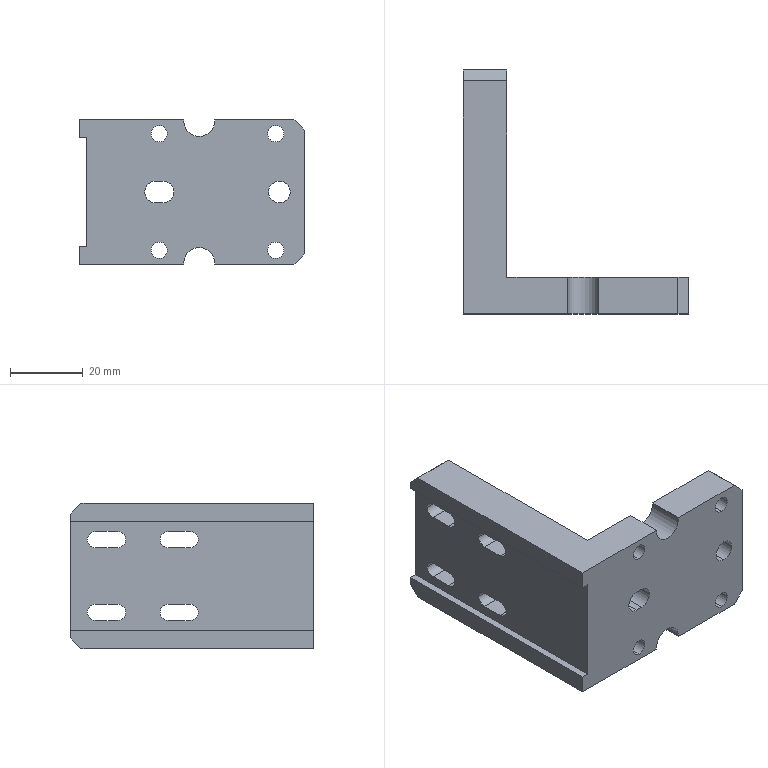Part | SolidWorks | features ICE 4, Chamfer 1, Cut 1, Extrusion 1, HoleWzd 1 | 1 solid | 58 faces | box 62 x 67 x 40 mm | volume 44252 mm3 | plane 32 | cylinder 26 | commonest cylinder face diameters 4.5 x20 6 x4 8.5 x2